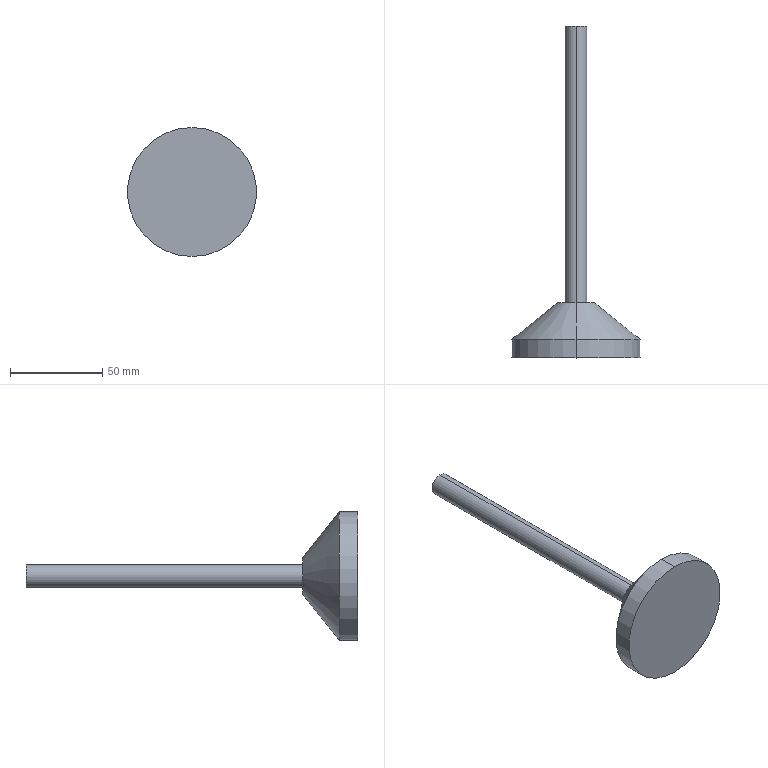Part | SolidWorks | features Chamfer 1, Extrusion 1, ICE 1 | 1 solid | 9 faces | box 70 x 180 x 70 mm | volume 90530 mm3 | cylinder 4 | plane 3 | cone 2 | commonest cylinder face diameters 12 x2 70 x2
STEP:
#1=CARTESIAN_POINT('',(0.,0.,10.));
#2=VERTEX_POINT('',#1);
#3=CARTESIAN_POINT('',(0.,0.,-10.));
#4=VERTEX_POINT('',#3);
#5=CARTESIAN_POINT('',(0.,0.,0.));
#6=DIRECTION('',(0.,1.,0.));
#7=DIRECTION('',(0.,0.,-1.));
#8=AXIS2_PLACEMENT_3D('',#5,#6,#7);
#9=CIRCLE('',#8,10.);
#10=EDGE_CURVE('',#2,#4,#9,.T.);
#11=ORIENTED_EDGE('',*,*,#10,.F.);
#12=CARTESIAN_POINT('',(0.,-20.,35.));
#13=VERTEX_POINT('',#12);
#14=CARTESIAN_POINT('',(0.,-20.,35.));
#15=DIRECTION('',(0.,-0.6247,0.7809));
#16=VECTOR('',#15,1000.);
#17=LINE('',#14,#16);
#18=EDGE_CURVE('',#2,#13,#17,.T.);
#19=ORIENTED_EDGE('',*,*,#18,.T.);
#20=CARTESIAN_POINT('',(0.,-20.,-35.));
#21=VERTEX_POINT('',#20);
#22=CARTESIAN_POINT('',(0.,-20.,0.));
#23=DIRECTION('',(0.,-1.,0.));
#24=DIRECTION('',(0.,0.,-1.));
#25=AXIS2_PLACEMENT_3D('',#22,#23,#24);
#26=CIRCLE('',#25,35.);
#27=EDGE_CURVE('',#21,#13,#26,.T.);
#28=ORIENTED_EDGE('',*,*,#27,.F.);
#29=CARTESIAN_POINT('',(0.,-20.,-35.));
#30=DIRECTION('',(0.,-0.6247,-0.7809));
#31=VECTOR('',#30,1000.);
#32=LINE('',#29,#31);
#33=EDGE_CURVE('',#4,#21,#32,.T.);
#34=ORIENTED_EDGE('',*,*,#33,.F.);
#35=EDGE_LOOP('',(#11,#19,#28,#34));
#36=FACE_OUTER_BOUND('',#35,.T.);
#37=CARTESIAN_POINT('',(0.,-20.,0.));
#38=DIRECTION('',(0.,-1.,0.));
#39=DIRECTION('',(0.,0.,-1.));
#40=AXIS2_PLACEMENT_3D('',#37,#38,#39);
#41=CONICAL_SURFACE('',#40,35.,0.8961);
#42=ADVANCED_FACE('',(#36),#41,.T.);
#43=CARTESIAN_POINT('',(0.,-30.,-35.));
#44=VERTEX_POINT('',#43);
#45=CARTESIAN_POINT('',(0.,-30.,35.));
#46=VERTEX_POINT('',#45);
#47=CARTESIAN_POINT('',(0.,-30.,0.));
#48=DIRECTION('',(0.,-1.,0.));
#49=DIRECTION('',(0.,0.,-1.));
#50=AXIS2_PLACEMENT_3D('',#47,#48,#49);
#51=CIRCLE('',#50,35.);
#52=EDGE_CURVE('',#44,#46,#51,.T.);
#53=ORIENTED_EDGE('',*,*,#52,.F.);
#54=CARTESIAN_POINT('',(0.,-30.,-35.));
#55=DIRECTION('',(0.,1.,0.));
#56=VECTOR('',#55,1000.);
#57=LINE('',#54,#56);
#58=EDGE_CURVE('',#44,#21,#57,.T.);
#59=ORIENTED_EDGE('',*,*,#58,.T.);
#60=ORIENTED_EDGE('',*,*,#27,.T.);
#61=CARTESIAN_POINT('',(0.,-30.,35.));
#62=DIRECTION('',(0.,1.,0.));
#63=VECTOR('',#62,1000.);
#64=LINE('',#61,#63);
#65=EDGE_CURVE('',#46,#13,#64,.T.);
#66=ORIENTED_EDGE('',*,*,#65,.F.);
#67=EDGE_LOOP('',(#53,#59,#60,#66));
#68=FACE_OUTER_BOUND('',#67,.T.);
#69=CARTESIAN_POINT('',(0.,-30.,0.));
#70=DIRECTION('',(0.,1.,0.));
#71=DIRECTION('',(0.,0.,1.));
#72=AXIS2_PLACEMENT_3D('',#69,#70,#71);
#73=CYLINDRICAL_SURFACE('',#72,35.);
#74=ADVANCED_FACE('',(#68),#73,.T.);
#75=CARTESIAN_POINT('',(0.,150.,6.));
#76=VERTEX_POINT('',#75);
#77=CARTESIAN_POINT('',(0.,150.,-6.));
#78=VERTEX_POINT('',#77);
#79=CARTESIAN_POINT('',(0.,150.,0.));
#80=DIRECTION('',(0.,1.,0.));
#81=DIRECTION('',(0.,0.,1.));
#82=AXIS2_PLACEMENT_3D('',#79,#80,#81);
#83=CIRCLE('',#82,6.);
#84=EDGE_CURVE('',#76,#78,#83,.T.);
#85=ORIENTED_EDGE('',*,*,#84,.F.);
#86=CARTESIAN_POINT('',(0.,0.,6.));
#87=VERTEX_POINT('',#86);
#88=CARTESIAN_POINT('',(0.,150.,6.));
#89=DIRECTION('',(0.,-1.,0.));
#90=VECTOR('',#89,1000.);
#91=LINE('',#88,#90);
#92=EDGE_CURVE('',#76,#87,#91,.T.);
#93=ORIENTED_EDGE('',*,*,#92,.T.);
#94=CARTESIAN_POINT('',(0.,0.,-6.));
#95=VERTEX_POINT('',#94);
#96=CARTESIAN_POINT('',(0.,0.,0.));
#97=DIRECTION('',(0.,-1.,0.));
#98=DIRECTION('',(0.,0.,-1.));
#99=AXIS2_PLACEMENT_3D('',#96,#97,#98);
#100=CIRCLE('',#99,6.);
#101=EDGE_CURVE('',#95,#87,#100,.T.);
#102=ORIENTED_EDGE('',*,*,#101,.F.);
#103=CARTESIAN_POINT('',(0.,150.,-6.));
#104=DIRECTION('',(0.,-1.,0.));
#105=VECTOR('',#104,1000.);
#106=LINE('',#103,#105);
#107=EDGE_CURVE('',#78,#95,#106,.T.);
#108=ORIENTED_EDGE('',*,*,#107,.F.);
#109=EDGE_LOOP('',(#85,#93,#102,#108));
#110=FACE_OUTER_BOUND('',#109,.T.);
#111=CARTESIAN_POINT('',(0.,150.,0.));
#112=DIRECTION('',(0.,-1.,0.));
#113=DIRECTION('',(0.,0.,-1.));
#114=AXIS2_PLACEMENT_3D('',#111,#112,#113);
#115=CYLINDRICAL_SURFACE('',#114,6.);
#116=ADVANCED_FACE('',(#110),#115,.T.);
#117=ORIENTED_EDGE('',*,*,#92,.F.);
#118=CARTESIAN_POINT('',(0.,150.,0.));
#119=DIRECTION('',(0.,1.,0.));
#120=DIRECTION('',(0.,0.,1.));
#121=AXIS2_PLACEMENT_3D('',#118,#119,#120);
#122=CIRCLE('',#121,6.);
#123=EDGE_CURVE('',#78,#76,#122,.T.);
#124=ORIENTED_EDGE('',*,*,#123,.F.);
#125=ORIENTED_EDGE('',*,*,#107,.T.);
#126=CARTESIAN_POINT('',(0.,0.,0.));
#127=DIRECTION('',(0.,-1.,0.));
#128=DIRECTION('',(0.,0.,-1.));
#129=AXIS2_PLACEMENT_3D('',#126,#127,#128);
#130=CIRCLE('',#129,6.);
#131=EDGE_CURVE('',#87,#95,#130,.T.);
#132=ORIENTED_EDGE('',*,*,#131,.F.);
#133=EDGE_LOOP('',(#117,#124,#125,#132));
#134=FACE_OUTER_BOUND('',#133,.T.);
#135=CARTESIAN_POINT('',(0.,150.,0.));
#136=DIRECTION('',(0.,-1.,0.));
#137=DIRECTION('',(0.,0.,-1.));
#138=AXIS2_PLACEMENT_3D('',#135,#136,#137);
#139=CYLINDRICAL_SURFACE('',#138,6.);
#140=ADVANCED_FACE('',(#134),#139,.T.);
#141=ORIENTED_EDGE('',*,*,#123,.T.);
#142=ORIENTED_EDGE('',*,*,#84,.T.);
#143=EDGE_LOOP('',(#141,#142));
#144=FACE_OUTER_BOUND('',#143,.T.);
#145=CARTESIAN_POINT('',(0.,150.,0.));
#146=DIRECTION('',(0.,1.,0.));
#147=DIRECTION('',(0.,0.,1.));
#148=AXIS2_PLACEMENT_3D('',#145,#146,#147);
#149=PLANE('',#148);
#150=ADVANCED_FACE('',(#144),#149,.T.);
#151=ORIENTED_EDGE('',*,*,#58,.F.);
#152=CARTESIAN_POINT('',(0.,-30.,0.));
#153=DIRECTION('',(0.,-1.,0.));
#154=DIRECTION('',(0.,0.,-1.));
#155=AXIS2_PLACEMENT_3D('',#152,#153,#154);
#156=CIRCLE('',#155,35.);
#157=EDGE_CURVE('',#46,#44,#156,.T.);
#158=ORIENTED_EDGE('',*,*,#157,.F.);
#159=ORIENTED_EDGE('',*,*,#65,.T.);
#160=CARTESIAN_POINT('',(0.,-20.,0.));
#161=DIRECTION('',(0.,-1.,0.));
#162=DIRECTION('',(0.,0.,-1.));
#163=AXIS2_PLACEMENT_3D('',#160,#161,#162);
#164=CIRCLE('',#163,35.);
#165=EDGE_CURVE('',#13,#21,#164,.T.);
#166=ORIENTED_EDGE('',*,*,#165,.T.);
#167=EDGE_LOOP('',(#151,#158,#159,#166));
#168=FACE_OUTER_BOUND('',#167,.T.);
#169=CARTESIAN_POINT('',(0.,-30.,0.));
#170=DIRECTION('',(0.,1.,0.));
#171=DIRECTION('',(0.,0.,1.));
#172=AXIS2_PLACEMENT_3D('',#169,#170,#171);
#173=CYLINDRICAL_SURFACE('',#172,35.);
#174=ADVANCED_FACE('',(#168),#173,.T.);
#175=ORIENTED_EDGE('',*,*,#157,.T.);
#176=ORIENTED_EDGE('',*,*,#52,.T.);
#177=EDGE_LOOP('',(#175,#176));
#178=FACE_OUTER_BOUND('',#177,.T.);
#179=CARTESIAN_POINT('',(0.,-30.,0.));
#180=DIRECTION('',(0.,-1.,0.));
#181=DIRECTION('',(0.,0.,-1.));
#182=AXIS2_PLACEMENT_3D('',#179,#180,#181);
#183=PLANE('',#182);
#184=ADVANCED_FACE('',(#178),#183,.T.);
#185=CARTESIAN_POINT('',(0.,0.,0.));
#186=DIRECTION('',(0.,1.,0.));
#187=DIRECTION('',(0.,0.,-1.));
#188=AXIS2_PLACEMENT_3D('',#185,#186,#187);
#189=CIRCLE('',#188,10.);
#190=EDGE_CURVE('',#4,#2,#189,.T.);
#191=ORIENTED_EDGE('',*,*,#190,.T.);
#192=ORIENTED_EDGE('',*,*,#10,.T.);
#193=EDGE_LOOP('',(#191,#192));
#194=FACE_OUTER_BOUND('',#193,.T.);
#195=ORIENTED_EDGE('',*,*,#101,.T.);
#196=ORIENTED_EDGE('',*,*,#131,.T.);
#197=EDGE_LOOP('',(#195,#196));
#198=FACE_BOUND('',#197,.T.);
#199=CARTESIAN_POINT('',(0.,0.,0.));
#200=DIRECTION('',(0.,-1.,0.));
#201=DIRECTION('',(0.,0.,-1.));
#202=AXIS2_PLACEMENT_3D('',#199,#200,#201);
#203=PLANE('',#202);
#204=ADVANCED_FACE('',(#194,#198),#203,.F.);
#205=ORIENTED_EDGE('',*,*,#18,.F.);
#206=ORIENTED_EDGE('',*,*,#190,.F.);
#207=ORIENTED_EDGE('',*,*,#33,.T.);
#208=ORIENTED_EDGE('',*,*,#165,.F.);
#209=EDGE_LOOP('',(#205,#206,#207,#208));
#210=FACE_OUTER_BOUND('',#209,.T.);
#211=CARTESIAN_POINT('',(0.,-20.,0.));
#212=DIRECTION('',(0.,-1.,0.));
#213=DIRECTION('',(0.,0.,-1.));
#214=AXIS2_PLACEMENT_3D('',#211,#212,#213);
#215=CONICAL_SURFACE('',#214,35.,0.8961);
#216=ADVANCED_FACE('',(#210),#215,.T.);
#217=CLOSED_SHELL('',(#42,#74,#116,#140,#150,#174,#184,#204,#216));
#218=MANIFOLD_SOLID_BREP('',#217);
#219=CARTESIAN_POINT('',(0.,0.,0.));
#220=DIRECTION('',(0.,0.,1.));
#221=DIRECTION('',(1.,0.,0.));
#222=AXIS2_PLACEMENT_3D('',#219,#220,#221);
#223=(LENGTH_UNIT()NAMED_UNIT(*)SI_UNIT(.MILLI.,.METRE.));
#224=UNCERTAINTY_MEASURE_WITH_UNIT(LENGTH_MEASURE(0.00001),#223,'','');
#225=(NAMED_UNIT(*)PLANE_ANGLE_UNIT()SI_UNIT($,.RADIAN.));
#226=(NAMED_UNIT(*)SI_UNIT($,.STERADIAN.)SOLID_ANGLE_UNIT());
#227=(GEOMETRIC_REPRESENTATION_CONTEXT(3)GLOBAL_UNCERTAINTY_ASSIGNED_CONTEXT((#224))GLOBAL_UNIT_ASSIGNED_CONTEXT((#223,#225,#226))REPRESENTATION_CONTEXT('',''));
#228=ADVANCED_BREP_SHAPE_REPRESENTATION('',(#218,#222),#227);